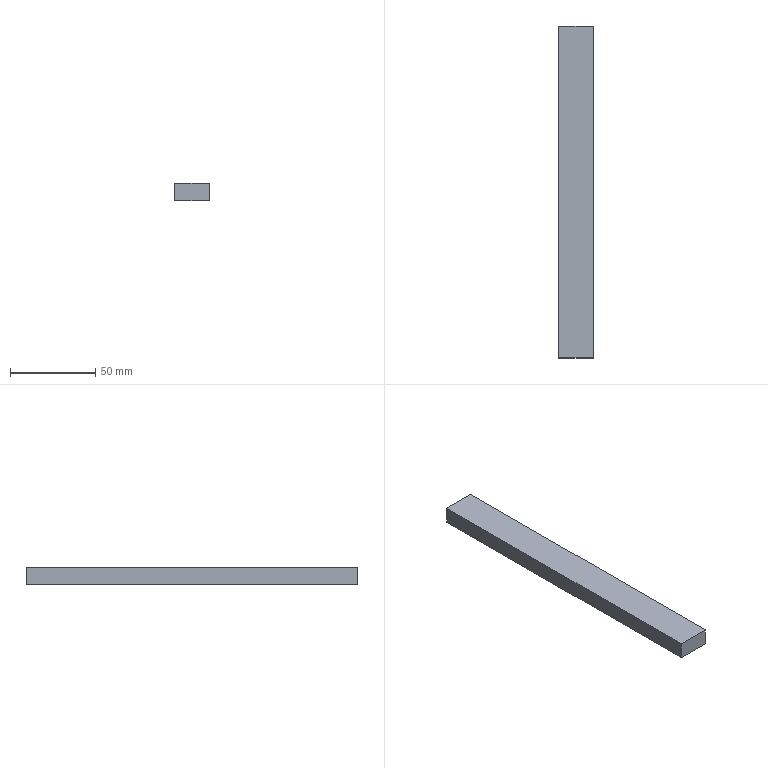Part | SolidWorks | features Extrusion 1 | 1 solid | 6 faces | box 20 x 195 x 10 mm | volume 39000 mm3 | plane 6
STEP:
#1=CARTESIAN_POINT('',(10.,-97.5,0.));
#2=VERTEX_POINT('',#1);
#3=CARTESIAN_POINT('',(10.,97.5,0.));
#4=VERTEX_POINT('',#3);
#5=CARTESIAN_POINT('',(10.,-97.5,0.));
#6=DIRECTION('',(0.,1.,0.));
#7=VECTOR('',#6,1000.);
#8=LINE('',#5,#7);
#9=EDGE_CURVE('',#2,#4,#8,.T.);
#10=ORIENTED_EDGE('',*,*,#9,.T.);
#11=CARTESIAN_POINT('',(10.,97.5,10.));
#12=VERTEX_POINT('',#11);
#13=CARTESIAN_POINT('',(10.,97.5,10.));
#14=DIRECTION('',(0.,0.,-1.));
#15=VECTOR('',#14,1000.);
#16=LINE('',#13,#15);
#17=EDGE_CURVE('',#12,#4,#16,.T.);
#18=ORIENTED_EDGE('',*,*,#17,.F.);
#19=CARTESIAN_POINT('',(10.,-97.5,10.));
#20=VERTEX_POINT('',#19);
#21=CARTESIAN_POINT('',(10.,-97.5,10.));
#22=DIRECTION('',(0.,1.,0.));
#23=VECTOR('',#22,1000.);
#24=LINE('',#21,#23);
#25=EDGE_CURVE('',#20,#12,#24,.T.);
#26=ORIENTED_EDGE('',*,*,#25,.F.);
#27=CARTESIAN_POINT('',(10.,-97.5,10.));
#28=DIRECTION('',(0.,0.,-1.));
#29=VECTOR('',#28,1000.);
#30=LINE('',#27,#29);
#31=EDGE_CURVE('',#20,#2,#30,.T.);
#32=ORIENTED_EDGE('',*,*,#31,.T.);
#33=EDGE_LOOP('',(#10,#18,#26,#32));
#34=FACE_OUTER_BOUND('',#33,.T.);
#35=CARTESIAN_POINT('',(10.,-97.5,10.));
#36=DIRECTION('',(-1.,0.,0.));
#37=DIRECTION('',(0.,0.,1.));
#38=AXIS2_PLACEMENT_3D('',#35,#36,#37);
#39=PLANE('',#38);
#40=ADVANCED_FACE('',(#34),#39,.F.);
#41=CARTESIAN_POINT('',(-10.,97.5,0.));
#42=VERTEX_POINT('',#41);
#43=CARTESIAN_POINT('',(-10.,97.5,0.));
#44=DIRECTION('',(-1.,0.,0.));
#45=VECTOR('',#44,1000.);
#46=LINE('',#43,#45);
#47=EDGE_CURVE('',#4,#42,#46,.T.);
#48=ORIENTED_EDGE('',*,*,#47,.T.);
#49=CARTESIAN_POINT('',(-10.,97.5,10.));
#50=VERTEX_POINT('',#49);
#51=CARTESIAN_POINT('',(-10.,97.5,10.));
#52=DIRECTION('',(0.,0.,-1.));
#53=VECTOR('',#52,1000.);
#54=LINE('',#51,#53);
#55=EDGE_CURVE('',#50,#42,#54,.T.);
#56=ORIENTED_EDGE('',*,*,#55,.F.);
#57=CARTESIAN_POINT('',(-10.,97.5,10.));
#58=DIRECTION('',(-1.,0.,0.));
#59=VECTOR('',#58,1000.);
#60=LINE('',#57,#59);
#61=EDGE_CURVE('',#12,#50,#60,.T.);
#62=ORIENTED_EDGE('',*,*,#61,.F.);
#63=ORIENTED_EDGE('',*,*,#17,.T.);
#64=EDGE_LOOP('',(#48,#56,#62,#63));
#65=FACE_OUTER_BOUND('',#64,.T.);
#66=CARTESIAN_POINT('',(-10.,97.5,10.));
#67=DIRECTION('',(0.,-1.,0.));
#68=DIRECTION('',(0.,0.,-1.));
#69=AXIS2_PLACEMENT_3D('',#66,#67,#68);
#70=PLANE('',#69);
#71=ADVANCED_FACE('',(#65),#70,.F.);
#72=CARTESIAN_POINT('',(-10.,-97.5,0.));
#73=VERTEX_POINT('',#72);
#74=CARTESIAN_POINT('',(-10.,-97.5,0.));
#75=DIRECTION('',(0.,-1.,0.));
#76=VECTOR('',#75,1000.);
#77=LINE('',#74,#76);
#78=EDGE_CURVE('',#42,#73,#77,.T.);
#79=ORIENTED_EDGE('',*,*,#78,.T.);
#80=CARTESIAN_POINT('',(-10.,-97.5,10.));
#81=VERTEX_POINT('',#80);
#82=CARTESIAN_POINT('',(-10.,-97.5,10.));
#83=DIRECTION('',(0.,0.,-1.));
#84=VECTOR('',#83,1000.);
#85=LINE('',#82,#84);
#86=EDGE_CURVE('',#81,#73,#85,.T.);
#87=ORIENTED_EDGE('',*,*,#86,.F.);
#88=CARTESIAN_POINT('',(-10.,-97.5,10.));
#89=DIRECTION('',(0.,-1.,0.));
#90=VECTOR('',#89,1000.);
#91=LINE('',#88,#90);
#92=EDGE_CURVE('',#50,#81,#91,.T.);
#93=ORIENTED_EDGE('',*,*,#92,.F.);
#94=ORIENTED_EDGE('',*,*,#55,.T.);
#95=EDGE_LOOP('',(#79,#87,#93,#94));
#96=FACE_OUTER_BOUND('',#95,.T.);
#97=CARTESIAN_POINT('',(-10.,-97.5,10.));
#98=DIRECTION('',(1.,0.,0.));
#99=DIRECTION('',(0.,0.,-1.));
#100=AXIS2_PLACEMENT_3D('',#97,#98,#99);
#101=PLANE('',#100);
#102=ADVANCED_FACE('',(#96),#101,.F.);
#103=CARTESIAN_POINT('',(-10.,-97.5,0.));
#104=DIRECTION('',(1.,0.,0.));
#105=VECTOR('',#104,1000.);
#106=LINE('',#103,#105);
#107=EDGE_CURVE('',#73,#2,#106,.T.);
#108=ORIENTED_EDGE('',*,*,#107,.T.);
#109=ORIENTED_EDGE('',*,*,#31,.F.);
#110=CARTESIAN_POINT('',(-10.,-97.5,10.));
#111=DIRECTION('',(1.,0.,0.));
#112=VECTOR('',#111,1000.);
#113=LINE('',#110,#112);
#114=EDGE_CURVE('',#81,#20,#113,.T.);
#115=ORIENTED_EDGE('',*,*,#114,.F.);
#116=ORIENTED_EDGE('',*,*,#86,.T.);
#117=EDGE_LOOP('',(#108,#109,#115,#116));
#118=FACE_OUTER_BOUND('',#117,.T.);
#119=CARTESIAN_POINT('',(-10.,-97.5,10.));
#120=DIRECTION('',(0.,1.,0.));
#121=DIRECTION('',(0.,0.,1.));
#122=AXIS2_PLACEMENT_3D('',#119,#120,#121);
#123=PLANE('',#122);
#124=ADVANCED_FACE('',(#118),#123,.F.);
#125=ORIENTED_EDGE('',*,*,#25,.T.);
#126=ORIENTED_EDGE('',*,*,#61,.T.);
#127=ORIENTED_EDGE('',*,*,#92,.T.);
#128=ORIENTED_EDGE('',*,*,#114,.T.);
#129=EDGE_LOOP('',(#125,#126,#127,#128));
#130=FACE_OUTER_BOUND('',#129,.T.);
#131=CARTESIAN_POINT('',(0.,0.,10.));
#132=DIRECTION('',(0.,0.,-1.));
#133=DIRECTION('',(-1.,0.,0.));
#134=AXIS2_PLACEMENT_3D('',#131,#132,#133);
#135=PLANE('',#134);
#136=ADVANCED_FACE('',(#130),#135,.F.);
#137=ORIENTED_EDGE('',*,*,#9,.F.);
#138=ORIENTED_EDGE('',*,*,#107,.F.);
#139=ORIENTED_EDGE('',*,*,#78,.F.);
#140=ORIENTED_EDGE('',*,*,#47,.F.);
#141=EDGE_LOOP('',(#137,#138,#139,#140));
#142=FACE_OUTER_BOUND('',#141,.T.);
#143=CARTESIAN_POINT('',(0.,0.,0.));
#144=DIRECTION('',(0.,0.,-1.));
#145=DIRECTION('',(-1.,0.,0.));
#146=AXIS2_PLACEMENT_3D('',#143,#144,#145);
#147=PLANE('',#146);
#148=ADVANCED_FACE('',(#142),#147,.T.);
#149=CLOSED_SHELL('',(#40,#71,#102,#124,#136,#148));
#150=MANIFOLD_SOLID_BREP('',#149);
#151=CARTESIAN_POINT('',(0.,0.,0.));
#152=DIRECTION('',(0.,0.,1.));
#153=DIRECTION('',(1.,0.,0.));
#154=AXIS2_PLACEMENT_3D('',#151,#152,#153);
#155=(LENGTH_UNIT()NAMED_UNIT(*)SI_UNIT(.MILLI.,.METRE.));
#156=UNCERTAINTY_MEASURE_WITH_UNIT(LENGTH_MEASURE(0.00001),#155,'','');
#157=(NAMED_UNIT(*)PLANE_ANGLE_UNIT()SI_UNIT($,.RADIAN.));
#158=(NAMED_UNIT(*)SI_UNIT($,.STERADIAN.)SOLID_ANGLE_UNIT());
#159=(GEOMETRIC_REPRESENTATION_CONTEXT(3)GLOBAL_UNCERTAINTY_ASSIGNED_CONTEXT((#156))GLOBAL_UNIT_ASSIGNED_CONTEXT((#155,#157,#158))REPRESENTATION_CONTEXT('',''));
#160=ADVANCED_BREP_SHAPE_REPRESENTATION('',(#150,#154),#159);